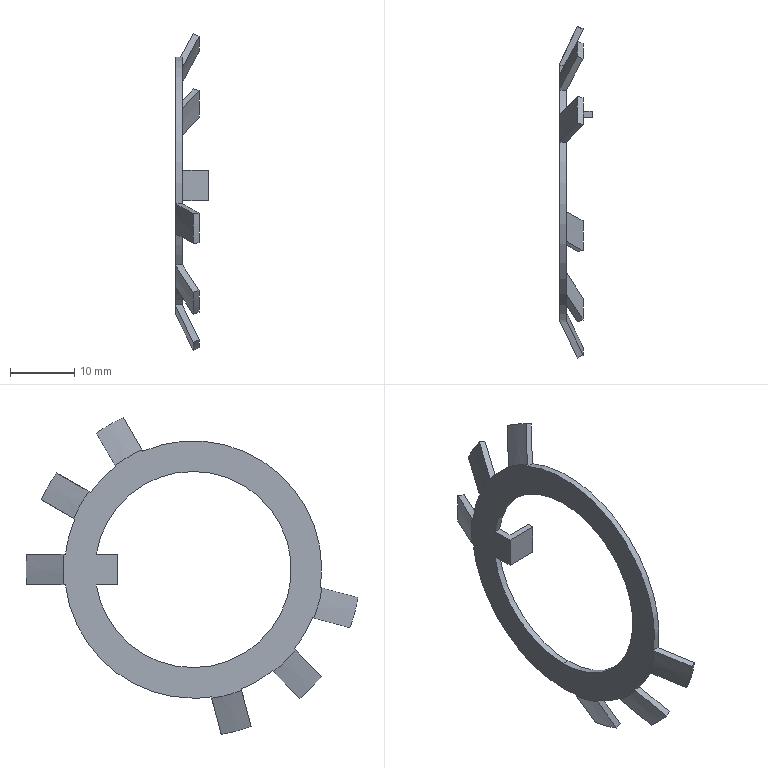Part | SolidWorks | features BaseBody 1 | 1 solid | 47 faces | box 5 x 51.628 x 49.249 mm | volume 745.679 mm3 | plane 19 | cone 18 | cylinder 10 | commonest cylinder face diameters 40 x7 30.5 x3